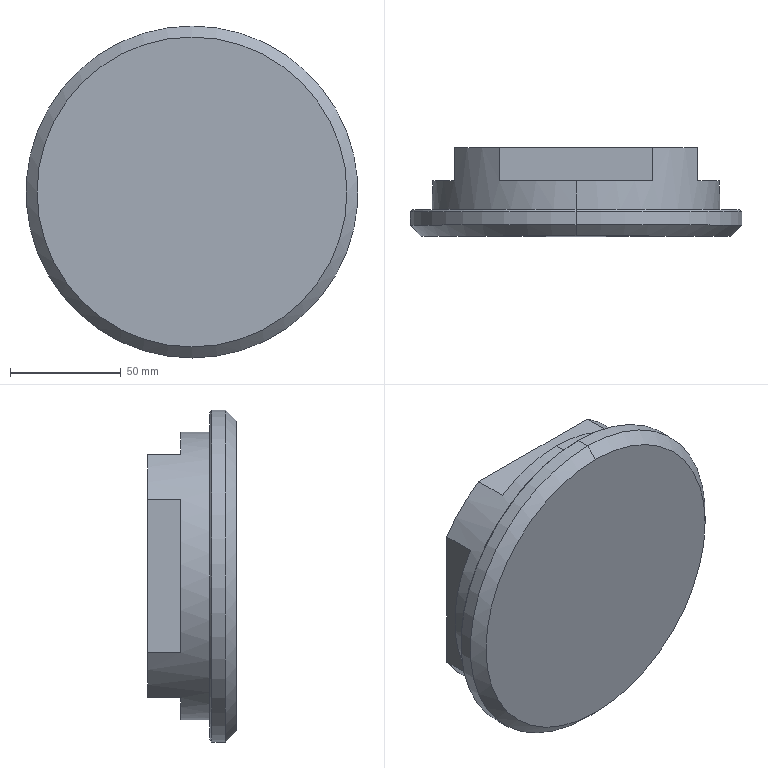Part | SolidWorks | features ICE 3, Chamfer 2, BaseBody 1 | 1 solid | 19 faces | box 150 x 40 x 150 mm | volume 549544 mm3 | plane 11 | cone 4 | cylinder 4 | commonest cylinder face diameters 130 x2 150 x2
STEP:
#1=CARTESIAN_POINT('',(0.,12.,74.));
#2=VERTEX_POINT('',#1);
#3=CARTESIAN_POINT('',(0.,12.,-74.));
#4=VERTEX_POINT('',#3);
#5=CARTESIAN_POINT('',(0.,12.,0.));
#6=DIRECTION('',(0.,1.,0.));
#7=DIRECTION('',(0.,0.,1.));
#8=AXIS2_PLACEMENT_3D('',#5,#6,#7);
#9=CIRCLE('',#8,74.);
#10=EDGE_CURVE('',#2,#4,#9,.T.);
#11=ORIENTED_EDGE('',*,*,#10,.F.);
#12=CARTESIAN_POINT('',(0.,11.,75.));
#13=VERTEX_POINT('',#12);
#14=CARTESIAN_POINT('',(0.,11.,75.));
#15=DIRECTION('',(0.,-0.7071,0.7071));
#16=VECTOR('',#15,1000.);
#17=LINE('',#14,#16);
#18=EDGE_CURVE('',#2,#13,#17,.T.);
#19=ORIENTED_EDGE('',*,*,#18,.T.);
#20=CARTESIAN_POINT('',(0.,11.,-75.));
#21=VERTEX_POINT('',#20);
#22=CARTESIAN_POINT('',(0.,11.,0.));
#23=DIRECTION('',(0.,-1.,0.));
#24=DIRECTION('',(0.,0.,1.));
#25=AXIS2_PLACEMENT_3D('',#22,#23,#24);
#26=CIRCLE('',#25,75.);
#27=EDGE_CURVE('',#21,#13,#26,.T.);
#28=ORIENTED_EDGE('',*,*,#27,.F.);
#29=CARTESIAN_POINT('',(0.,11.,-75.));
#30=DIRECTION('',(0.,-0.7071,-0.7071));
#31=VECTOR('',#30,1000.);
#32=LINE('',#29,#31);
#33=EDGE_CURVE('',#4,#21,#32,.T.);
#34=ORIENTED_EDGE('',*,*,#33,.F.);
#35=EDGE_LOOP('',(#11,#19,#28,#34));
#36=FACE_OUTER_BOUND('',#35,.T.);
#37=CARTESIAN_POINT('',(0.,11.,0.));
#38=DIRECTION('',(0.,-1.,0.));
#39=DIRECTION('',(0.,0.,-1.));
#40=AXIS2_PLACEMENT_3D('',#37,#38,#39);
#41=CONICAL_SURFACE('',#40,75.,0.7854);
#42=ADVANCED_FACE('',(#36),#41,.T.);
#43=CARTESIAN_POINT('',(0.,0.,-70.));
#44=VERTEX_POINT('',#43);
#45=CARTESIAN_POINT('',(0.,0.,70.));
#46=VERTEX_POINT('',#45);
#47=CARTESIAN_POINT('',(0.,0.,0.));
#48=DIRECTION('',(0.,-1.,0.));
#49=DIRECTION('',(0.,0.,1.));
#50=AXIS2_PLACEMENT_3D('',#47,#48,#49);
#51=CIRCLE('',#50,70.);
#52=EDGE_CURVE('',#44,#46,#51,.T.);
#53=ORIENTED_EDGE('',*,*,#52,.F.);
#54=CARTESIAN_POINT('',(0.,5.,-75.));
#55=VERTEX_POINT('',#54);
#56=CARTESIAN_POINT('',(0.,0.,-70.));
#57=DIRECTION('',(0.,0.7071,-0.7071));
#58=VECTOR('',#57,1000.);
#59=LINE('',#56,#58);
#60=EDGE_CURVE('',#44,#55,#59,.T.);
#61=ORIENTED_EDGE('',*,*,#60,.T.);
#62=CARTESIAN_POINT('',(0.,5.,75.));
#63=VERTEX_POINT('',#62);
#64=CARTESIAN_POINT('',(0.,5.,0.));
#65=DIRECTION('',(0.,1.,0.));
#66=DIRECTION('',(0.,0.,1.));
#67=AXIS2_PLACEMENT_3D('',#64,#65,#66);
#68=CIRCLE('',#67,75.);
#69=EDGE_CURVE('',#63,#55,#68,.T.);
#70=ORIENTED_EDGE('',*,*,#69,.F.);
#71=CARTESIAN_POINT('',(0.,0.,70.));
#72=DIRECTION('',(0.,0.7071,0.7071));
#73=VECTOR('',#72,1000.);
#74=LINE('',#71,#73);
#75=EDGE_CURVE('',#46,#63,#74,.T.);
#76=ORIENTED_EDGE('',*,*,#75,.F.);
#77=EDGE_LOOP('',(#53,#61,#70,#76));
#78=FACE_OUTER_BOUND('',#77,.T.);
#79=CARTESIAN_POINT('',(0.,0.,0.));
#80=DIRECTION('',(0.,1.,0.));
#81=DIRECTION('',(0.,0.,1.));
#82=AXIS2_PLACEMENT_3D('',#79,#80,#81);
#83=CONICAL_SURFACE('',#82,70.,0.7854);
#84=ADVANCED_FACE('',(#78),#83,.T.);
#85=ORIENTED_EDGE('',*,*,#27,.T.);
#86=CARTESIAN_POINT('',(0.,224.132,75.));
#87=DIRECTION('',(0.,-1.,0.));
#88=VECTOR('',#87,1000.);
#89=LINE('',#86,#88);
#90=EDGE_CURVE('',#13,#63,#89,.T.);
#91=ORIENTED_EDGE('',*,*,#90,.T.);
#92=ORIENTED_EDGE('',*,*,#69,.T.);
#93=CARTESIAN_POINT('',(0.,224.132,-75.));
#94=DIRECTION('',(0.,-1.,0.));
#95=VECTOR('',#94,1000.);
#96=LINE('',#93,#95);
#97=EDGE_CURVE('',#21,#55,#96,.T.);
#98=ORIENTED_EDGE('',*,*,#97,.F.);
#99=EDGE_LOOP('',(#85,#91,#92,#98));
#100=FACE_OUTER_BOUND('',#99,.T.);
#101=CARTESIAN_POINT('',(0.,224.132,0.));
#102=DIRECTION('',(0.,-1.,0.));
#103=DIRECTION('',(0.,0.,-1.));
#104=AXIS2_PLACEMENT_3D('',#101,#102,#103);
#105=CYLINDRICAL_SURFACE('',#104,75.);
#106=ADVANCED_FACE('',(#100),#105,.T.);
#107=CARTESIAN_POINT('',(0.,25.,65.));
#108=VERTEX_POINT('',#107);
#109=CARTESIAN_POINT('',(34.641,25.,55.));
#110=VERTEX_POINT('',#109);
#111=CARTESIAN_POINT('',(0.,25.,0.));
#112=DIRECTION('',(0.,1.,0.));
#113=DIRECTION('',(0.,0.,1.));
#114=AXIS2_PLACEMENT_3D('',#111,#112,#113);
#115=CIRCLE('',#114,65.);
#116=EDGE_CURVE('',#108,#110,#115,.T.);
#117=ORIENTED_EDGE('',*,*,#116,.F.);
#118=CARTESIAN_POINT('',(0.,12.,65.));
#119=VERTEX_POINT('',#118);
#120=CARTESIAN_POINT('',(0.,208.848,65.));
#121=DIRECTION('',(0.,-1.,0.));
#122=VECTOR('',#121,1000.);
#123=LINE('',#120,#122);
#124=EDGE_CURVE('',#108,#119,#123,.T.);
#125=ORIENTED_EDGE('',*,*,#124,.T.);
#126=CARTESIAN_POINT('',(0.,12.,-65.));
#127=VERTEX_POINT('',#126);
#128=CARTESIAN_POINT('',(0.,12.,0.));
#129=DIRECTION('',(0.,1.,0.));
#130=DIRECTION('',(0.,0.,1.));
#131=AXIS2_PLACEMENT_3D('',#128,#129,#130);
#132=CIRCLE('',#131,65.);
#133=EDGE_CURVE('',#119,#127,#132,.T.);
#134=ORIENTED_EDGE('',*,*,#133,.T.);
#135=CARTESIAN_POINT('',(0.,25.,-65.));
#136=VERTEX_POINT('',#135);
#137=CARTESIAN_POINT('',(0.,208.848,-65.));
#138=DIRECTION('',(0.,-1.,0.));
#139=VECTOR('',#138,1000.);
#140=LINE('',#137,#139);
#141=EDGE_CURVE('',#136,#127,#140,.T.);
#142=ORIENTED_EDGE('',*,*,#141,.F.);
#143=CARTESIAN_POINT('',(34.641,25.,-55.));
#144=VERTEX_POINT('',#143);
#145=CARTESIAN_POINT('',(0.,25.,0.));
#146=DIRECTION('',(0.,1.,0.));
#147=DIRECTION('',(0.,0.,1.));
#148=AXIS2_PLACEMENT_3D('',#145,#146,#147);
#149=CIRCLE('',#148,65.);
#150=EDGE_CURVE('',#144,#136,#149,.T.);
#151=ORIENTED_EDGE('',*,*,#150,.F.);
#152=CARTESIAN_POINT('',(34.641,40.,-55.));
#153=VERTEX_POINT('',#152);
#154=CARTESIAN_POINT('',(34.641,195.563,-55.));
#155=DIRECTION('',(0.,-1.,0.));
#156=VECTOR('',#155,1000.);
#157=LINE('',#154,#156);
#158=EDGE_CURVE('',#153,#144,#157,.T.);
#159=ORIENTED_EDGE('',*,*,#158,.F.);
#160=CARTESIAN_POINT('',(55.,40.,-34.641));
#161=VERTEX_POINT('',#160);
#162=CARTESIAN_POINT('',(0.,40.,0.));
#163=DIRECTION('',(0.,1.,0.));
#164=DIRECTION('',(0.,0.,1.));
#165=AXIS2_PLACEMENT_3D('',#162,#163,#164);
#166=CIRCLE('',#165,65.);
#167=EDGE_CURVE('',#161,#153,#166,.T.);
#168=ORIENTED_EDGE('',*,*,#167,.F.);
#169=CARTESIAN_POINT('',(55.,25.,-34.641));
#170=VERTEX_POINT('',#169);
#171=CARTESIAN_POINT('',(55.,195.563,-34.641));
#172=DIRECTION('',(0.,-1.,0.));
#173=VECTOR('',#172,1000.);
#174=LINE('',#171,#173);
#175=EDGE_CURVE('',#161,#170,#174,.T.);
#176=ORIENTED_EDGE('',*,*,#175,.T.);
#177=CARTESIAN_POINT('',(55.,25.,34.641));
#178=VERTEX_POINT('',#177);
#179=CARTESIAN_POINT('',(0.,25.,0.));
#180=DIRECTION('',(0.,1.,0.));
#181=DIRECTION('',(0.,0.,1.));
#182=AXIS2_PLACEMENT_3D('',#179,#180,#181);
#183=CIRCLE('',#182,65.);
#184=EDGE_CURVE('',#178,#170,#183,.T.);
#185=ORIENTED_EDGE('',*,*,#184,.F.);
#186=CARTESIAN_POINT('',(55.,40.,34.641));
#187=VERTEX_POINT('',#186);
#188=CARTESIAN_POINT('',(55.,195.563,34.641));
#189=DIRECTION('',(0.,-1.,0.));
#190=VECTOR('',#189,1000.);
#191=LINE('',#188,#190);
#192=EDGE_CURVE('',#187,#178,#191,.T.);
#193=ORIENTED_EDGE('',*,*,#192,.F.);
#194=CARTESIAN_POINT('',(34.641,40.,55.));
#195=VERTEX_POINT('',#194);
#196=CARTESIAN_POINT('',(0.,40.,0.));
#197=DIRECTION('',(0.,1.,0.));
#198=DIRECTION('',(0.,0.,1.));
#199=AXIS2_PLACEMENT_3D('',#196,#197,#198);
#200=CIRCLE('',#199,65.);
#201=EDGE_CURVE('',#195,#187,#200,.T.);
#202=ORIENTED_EDGE('',*,*,#201,.F.);
#203=CARTESIAN_POINT('',(34.641,195.563,55.));
#204=DIRECTION('',(0.,-1.,0.));
#205=VECTOR('',#204,1000.);
#206=LINE('',#203,#205);
#207=EDGE_CURVE('',#195,#110,#206,.T.);
#208=ORIENTED_EDGE('',*,*,#207,.T.);
#209=EDGE_LOOP('',(#117,#125,#134,#142,#151,#159,#168,#176,#185,#193,#202,#208));
#210=FACE_OUTER_BOUND('',#209,.T.);
#211=CARTESIAN_POINT('',(0.,208.848,0.));
#212=DIRECTION('',(0.,-1.,0.));
#213=DIRECTION('',(0.,0.,-1.));
#214=AXIS2_PLACEMENT_3D('',#211,#212,#213);
#215=CYLINDRICAL_SURFACE('',#214,65.);
#216=ADVANCED_FACE('',(#210),#215,.T.);
#217=CARTESIAN_POINT('',(-55.,25.,-34.641));
#218=VERTEX_POINT('',#217);
#219=CARTESIAN_POINT('',(-55.,25.,34.641));
#220=VERTEX_POINT('',#219);
#221=CARTESIAN_POINT('',(0.,25.,0.));
#222=DIRECTION('',(0.,1.,0.));
#223=DIRECTION('',(0.,0.,1.));
#224=AXIS2_PLACEMENT_3D('',#221,#222,#223);
#225=CIRCLE('',#224,65.);
#226=EDGE_CURVE('',#218,#220,#225,.T.);
#227=ORIENTED_EDGE('',*,*,#226,.T.);
#228=CARTESIAN_POINT('',(-55.,25.,34.641));
#229=DIRECTION('',(0.,0.,1.));
#230=VECTOR('',#229,1000.);
#231=LINE('',#228,#230);
#232=EDGE_CURVE('',#218,#220,#231,.T.);
#233=ORIENTED_EDGE('',*,*,#232,.F.);
#234=EDGE_LOOP('',(#227,#233));
#235=FACE_OUTER_BOUND('',#234,.T.);
#236=CARTESIAN_POINT('',(0.,25.,0.));
#237=DIRECTION('',(0.,1.,0.));
#238=DIRECTION('',(0.,0.,1.));
#239=AXIS2_PLACEMENT_3D('',#236,#237,#238);
#240=PLANE('',#239);
#241=ADVANCED_FACE('',(#235),#240,.T.);
#242=CARTESIAN_POINT('',(-34.641,25.,55.));
#243=VERTEX_POINT('',#242);
#244=CARTESIAN_POINT('',(0.,25.,0.));
#245=DIRECTION('',(0.,1.,0.));
#246=DIRECTION('',(0.,0.,1.));
#247=AXIS2_PLACEMENT_3D('',#244,#245,#246);
#248=CIRCLE('',#247,65.);
#249=EDGE_CURVE('',#243,#108,#248,.T.);
#250=ORIENTED_EDGE('',*,*,#249,.T.);
#251=ORIENTED_EDGE('',*,*,#116,.T.);
#252=CARTESIAN_POINT('',(-34.641,25.,55.));
#253=DIRECTION('',(1.,0.,0.));
#254=VECTOR('',#253,1000.);
#255=LINE('',#252,#254);
#256=EDGE_CURVE('',#243,#110,#255,.T.);
#257=ORIENTED_EDGE('',*,*,#256,.F.);
#258=EDGE_LOOP('',(#250,#251,#257));
#259=FACE_OUTER_BOUND('',#258,.T.);
#260=CARTESIAN_POINT('',(0.,25.,0.));
#261=DIRECTION('',(0.,1.,0.));
#262=DIRECTION('',(0.,0.,1.));
#263=AXIS2_PLACEMENT_3D('',#260,#261,#262);
#264=PLANE('',#263);
#265=ADVANCED_FACE('',(#259),#264,.T.);
#266=ORIENTED_EDGE('',*,*,#184,.T.);
#267=CARTESIAN_POINT('',(55.,25.,34.641));
#268=DIRECTION('',(0.,0.,-1.));
#269=VECTOR('',#268,1000.);
#270=LINE('',#267,#269);
#271=EDGE_CURVE('',#178,#170,#270,.T.);
#272=ORIENTED_EDGE('',*,*,#271,.F.);
#273=EDGE_LOOP('',(#266,#272));
#274=FACE_OUTER_BOUND('',#273,.T.);
#275=CARTESIAN_POINT('',(0.,25.,0.));
#276=DIRECTION('',(0.,1.,0.));
#277=DIRECTION('',(0.,0.,1.));
#278=AXIS2_PLACEMENT_3D('',#275,#276,#277);
#279=PLANE('',#278);
#280=ADVANCED_FACE('',(#274),#279,.T.);
#281=ORIENTED_EDGE('',*,*,#150,.T.);
#282=CARTESIAN_POINT('',(-34.641,25.,-55.));
#283=VERTEX_POINT('',#282);
#284=CARTESIAN_POINT('',(0.,25.,0.));
#285=DIRECTION('',(0.,1.,0.));
#286=DIRECTION('',(0.,0.,1.));
#287=AXIS2_PLACEMENT_3D('',#284,#285,#286);
#288=CIRCLE('',#287,65.);
#289=EDGE_CURVE('',#136,#283,#288,.T.);
#290=ORIENTED_EDGE('',*,*,#289,.T.);
#291=CARTESIAN_POINT('',(-34.641,25.,-55.));
#292=DIRECTION('',(-1.,0.,0.));
#293=VECTOR('',#292,1000.);
#294=LINE('',#291,#293);
#295=EDGE_CURVE('',#144,#283,#294,.T.);
#296=ORIENTED_EDGE('',*,*,#295,.F.);
#297=EDGE_LOOP('',(#281,#290,#296));
#298=FACE_OUTER_BOUND('',#297,.T.);
#299=CARTESIAN_POINT('',(0.,25.,0.));
#300=DIRECTION('',(0.,1.,0.));
#301=DIRECTION('',(0.,0.,1.));
#302=AXIS2_PLACEMENT_3D('',#299,#300,#301);
#303=PLANE('',#302);
#304=ADVANCED_FACE('',(#298),#303,.T.);
#305=ORIENTED_EDGE('',*,*,#124,.F.);
#306=ORIENTED_EDGE('',*,*,#249,.F.);
#307=CARTESIAN_POINT('',(-34.641,40.,55.));
#308=VERTEX_POINT('',#307);
#309=CARTESIAN_POINT('',(-34.641,195.563,55.));
#310=DIRECTION('',(0.,-1.,0.));
#311=VECTOR('',#310,1000.);
#312=LINE('',#309,#311);
#313=EDGE_CURVE('',#308,#243,#312,.T.);
#314=ORIENTED_EDGE('',*,*,#313,.F.);
#315=CARTESIAN_POINT('',(-55.,40.,34.641));
#316=VERTEX_POINT('',#315);
#317=CARTESIAN_POINT('',(0.,40.,0.));
#318=DIRECTION('',(0.,1.,0.));
#319=DIRECTION('',(0.,0.,1.));
#320=AXIS2_PLACEMENT_3D('',#317,#318,#319);
#321=CIRCLE('',#320,65.);
#322=EDGE_CURVE('',#316,#308,#321,.T.);
#323=ORIENTED_EDGE('',*,*,#322,.F.);
#324=CARTESIAN_POINT('',(-55.,195.563,34.641));
#325=DIRECTION('',(0.,-1.,0.));
#326=VECTOR('',#325,1000.);
#327=LINE('',#324,#326);
#328=EDGE_CURVE('',#316,#220,#327,.T.);
#329=ORIENTED_EDGE('',*,*,#328,.T.);
#330=ORIENTED_EDGE('',*,*,#226,.F.);
#331=CARTESIAN_POINT('',(-55.,40.,-34.641));
#332=VERTEX_POINT('',#331);
#333=CARTESIAN_POINT('',(-55.,195.563,-34.641));
#334=DIRECTION('',(0.,-1.,0.));
#335=VECTOR('',#334,1000.);
#336=LINE('',#333,#335);
#337=EDGE_CURVE('',#332,#218,#336,.T.);
#338=ORIENTED_EDGE('',*,*,#337,.F.);
#339=CARTESIAN_POINT('',(-34.641,40.,-55.));
#340=VERTEX_POINT('',#339);
#341=CARTESIAN_POINT('',(0.,40.,0.));
#342=DIRECTION('',(0.,1.,0.));
#343=DIRECTION('',(0.,0.,1.));
#344=AXIS2_PLACEMENT_3D('',#341,#342,#343);
#345=CIRCLE('',#344,65.);
#346=EDGE_CURVE('',#340,#332,#345,.T.);
#347=ORIENTED_EDGE('',*,*,#346,.F.);
#348=CARTESIAN_POINT('',(-34.641,195.563,-55.));
#349=DIRECTION('',(0.,-1.,0.));
#350=VECTOR('',#349,1000.);
#351=LINE('',#348,#350);
#352=EDGE_CURVE('',#340,#283,#351,.T.);
#353=ORIENTED_EDGE('',*,*,#352,.T.);
#354=ORIENTED_EDGE('',*,*,#289,.F.);
#355=ORIENTED_EDGE('',*,*,#141,.T.);
#356=CARTESIAN_POINT('',(0.,12.,0.));
#357=DIRECTION('',(0.,1.,0.));
#358=DIRECTION('',(0.,0.,1.));
#359=AXIS2_PLACEMENT_3D('',#356,#357,#358);
#360=CIRCLE('',#359,65.);
#361=EDGE_CURVE('',#127,#119,#360,.T.);
#362=ORIENTED_EDGE('',*,*,#361,.T.);
#363=EDGE_LOOP('',(#305,#306,#314,#323,#329,#330,#338,#347,#353,#354,#355,#362));
#364=FACE_OUTER_BOUND('',#363,.T.);
#365=CARTESIAN_POINT('',(0.,208.848,0.));
#366=DIRECTION('',(0.,-1.,0.));
#367=DIRECTION('',(0.,0.,-1.));
#368=AXIS2_PLACEMENT_3D('',#365,#366,#367);
#369=CYLINDRICAL_SURFACE('',#368,65.);
#370=ADVANCED_FACE('',(#364),#369,.T.);
#371=CARTESIAN_POINT('',(0.,12.,0.));
#372=DIRECTION('',(0.,1.,0.));
#373=DIRECTION('',(0.,0.,1.));
#374=AXIS2_PLACEMENT_3D('',#371,#372,#373);
#375=CIRCLE('',#374,74.);
#376=EDGE_CURVE('',#4,#2,#375,.T.);
#377=ORIENTED_EDGE('',*,*,#376,.T.);
#378=ORIENTED_EDGE('',*,*,#10,.T.);
#379=EDGE_LOOP('',(#377,#378));
#380=FACE_OUTER_BOUND('',#379,.T.);
#381=ORIENTED_EDGE('',*,*,#361,.F.);
#382=ORIENTED_EDGE('',*,*,#133,.F.);
#383=EDGE_LOOP('',(#381,#382));
#384=FACE_BOUND('',#383,.T.);
#385=CARTESIAN_POINT('',(0.,12.,0.));
#386=DIRECTION('',(0.,1.,0.));
#387=DIRECTION('',(0.,0.,1.));
#388=AXIS2_PLACEMENT_3D('',#385,#386,#387);
#389=PLANE('',#388);
#390=ADVANCED_FACE('',(#380,#384),#389,.T.);
#391=ORIENTED_EDGE('',*,*,#90,.F.);
#392=CARTESIAN_POINT('',(0.,11.,0.));
#393=DIRECTION('',(0.,-1.,0.));
#394=DIRECTION('',(0.,0.,1.));
#395=AXIS2_PLACEMENT_3D('',#392,#393,#394);
#396=CIRCLE('',#395,75.);
#397=EDGE_CURVE('',#13,#21,#396,.T.);
#398=ORIENTED_EDGE('',*,*,#397,.T.);
#399=ORIENTED_EDGE('',*,*,#97,.T.);
#400=CARTESIAN_POINT('',(0.,5.,0.));
#401=DIRECTION('',(0.,1.,0.));
#402=DIRECTION('',(0.,0.,1.));
#403=AXIS2_PLACEMENT_3D('',#400,#401,#402);
#404=CIRCLE('',#403,75.);
#405=EDGE_CURVE('',#55,#63,#404,.T.);
#406=ORIENTED_EDGE('',*,*,#405,.T.);
#407=EDGE_LOOP('',(#391,#398,#399,#406));
#408=FACE_OUTER_BOUND('',#407,.T.);
#409=CARTESIAN_POINT('',(0.,224.132,0.));
#410=DIRECTION('',(0.,-1.,0.));
#411=DIRECTION('',(0.,0.,-1.));
#412=AXIS2_PLACEMENT_3D('',#409,#410,#411);
#413=CYLINDRICAL_SURFACE('',#412,75.);
#414=ADVANCED_FACE('',(#408),#413,.T.);
#415=CARTESIAN_POINT('',(0.,0.,0.));
#416=DIRECTION('',(0.,-1.,0.));
#417=DIRECTION('',(0.,0.,1.));
#418=AXIS2_PLACEMENT_3D('',#415,#416,#417);
#419=CIRCLE('',#418,70.);
#420=EDGE_CURVE('',#46,#44,#419,.T.);
#421=ORIENTED_EDGE('',*,*,#420,.T.);
#422=ORIENTED_EDGE('',*,*,#52,.T.);
#423=EDGE_LOOP('',(#421,#422));
#424=FACE_OUTER_BOUND('',#423,.T.);
#425=CARTESIAN_POINT('',(0.,0.,0.));
#426=DIRECTION('',(0.,1.,0.));
#427=DIRECTION('',(0.,0.,1.));
#428=AXIS2_PLACEMENT_3D('',#425,#426,#427);
#429=PLANE('',#428);
#430=ADVANCED_FACE('',(#424),#429,.F.);
#431=CARTESIAN_POINT('',(-34.641,40.,-55.));
#432=DIRECTION('',(-1.,0.,0.));
#433=VECTOR('',#432,1000.);
#434=LINE('',#431,#433);
#435=EDGE_CURVE('',#153,#340,#434,.T.);
#436=ORIENTED_EDGE('',*,*,#435,.F.);
#437=ORIENTED_EDGE('',*,*,#158,.T.);
#438=ORIENTED_EDGE('',*,*,#295,.T.);
#439=ORIENTED_EDGE('',*,*,#352,.F.);
#440=EDGE_LOOP('',(#436,#437,#438,#439));
#441=FACE_OUTER_BOUND('',#440,.T.);
#442=CARTESIAN_POINT('',(-34.641,195.563,-55.));
#443=DIRECTION('',(0.,0.,1.));
#444=DIRECTION('',(1.,0.,0.));
#445=AXIS2_PLACEMENT_3D('',#442,#443,#444);
#446=PLANE('',#445);
#447=ADVANCED_FACE('',(#441),#446,.F.);
#448=CARTESIAN_POINT('',(55.,40.,34.641));
#449=DIRECTION('',(0.,0.,-1.));
#450=VECTOR('',#449,1000.);
#451=LINE('',#448,#450);
#452=EDGE_CURVE('',#187,#161,#451,.T.);
#453=ORIENTED_EDGE('',*,*,#452,.F.);
#454=ORIENTED_EDGE('',*,*,#192,.T.);
#455=ORIENTED_EDGE('',*,*,#271,.T.);
#456=ORIENTED_EDGE('',*,*,#175,.F.);
#457=EDGE_LOOP('',(#453,#454,#455,#456));
#458=FACE_OUTER_BOUND('',#457,.T.);
#459=CARTESIAN_POINT('',(55.,195.563,34.641));
#460=DIRECTION('',(-1.,0.,0.));
#461=DIRECTION('',(0.,0.,1.));
#462=AXIS2_PLACEMENT_3D('',#459,#460,#461);
#463=PLANE('',#462);
#464=ADVANCED_FACE('',(#458),#463,.F.);
#465=CARTESIAN_POINT('',(-34.641,40.,55.));
#466=DIRECTION('',(1.,0.,0.));
#467=VECTOR('',#466,1000.);
#468=LINE('',#465,#467);
#469=EDGE_CURVE('',#308,#195,#468,.T.);
#470=ORIENTED_EDGE('',*,*,#469,.F.);
#471=ORIENTED_EDGE('',*,*,#313,.T.);
#472=ORIENTED_EDGE('',*,*,#256,.T.);
#473=ORIENTED_EDGE('',*,*,#207,.F.);
#474=EDGE_LOOP('',(#470,#471,#472,#473));
#475=FACE_OUTER_BOUND('',#474,.T.);
#476=CARTESIAN_POINT('',(-34.641,195.563,55.));
#477=DIRECTION('',(0.,0.,-1.));
#478=DIRECTION('',(-1.,0.,0.));
#479=AXIS2_PLACEMENT_3D('',#476,#477,#478);
#480=PLANE('',#479);
#481=ADVANCED_FACE('',(#475),#480,.F.);
#482=CARTESIAN_POINT('',(-55.,40.,34.641));
#483=DIRECTION('',(0.,0.,1.));
#484=VECTOR('',#483,1000.);
#485=LINE('',#482,#484);
#486=EDGE_CURVE('',#332,#316,#485,.T.);
#487=ORIENTED_EDGE('',*,*,#486,.F.);
#488=ORIENTED_EDGE('',*,*,#337,.T.);
#489=ORIENTED_EDGE('',*,*,#232,.T.);
#490=ORIENTED_EDGE('',*,*,#328,.F.);
#491=EDGE_LOOP('',(#487,#488,#489,#490));
#492=FACE_OUTER_BOUND('',#491,.T.);
#493=CARTESIAN_POINT('',(-55.,195.563,34.641));
#494=DIRECTION('',(1.,0.,0.));
#495=DIRECTION('',(0.,0.,-1.));
#496=AXIS2_PLACEMENT_3D('',#493,#494,#495);
#497=PLANE('',#496);
#498=ADVANCED_FACE('',(#492),#497,.F.);
#499=ORIENTED_EDGE('',*,*,#435,.T.);
#500=ORIENTED_EDGE('',*,*,#346,.T.);
#501=ORIENTED_EDGE('',*,*,#486,.T.);
#502=ORIENTED_EDGE('',*,*,#322,.T.);
#503=ORIENTED_EDGE('',*,*,#469,.T.);
#504=ORIENTED_EDGE('',*,*,#201,.T.);
#505=ORIENTED_EDGE('',*,*,#452,.T.);
#506=ORIENTED_EDGE('',*,*,#167,.T.);
#507=EDGE_LOOP('',(#499,#500,#501,#502,#503,#504,#505,#506));
#508=FACE_OUTER_BOUND('',#507,.T.);
#509=CARTESIAN_POINT('',(0.,40.,0.));
#510=DIRECTION('',(0.,1.,0.));
#511=DIRECTION('',(0.,0.,1.));
#512=AXIS2_PLACEMENT_3D('',#509,#510,#511);
#513=PLANE('',#512);
#514=ADVANCED_FACE('',(#508),#513,.T.);
#515=ORIENTED_EDGE('',*,*,#60,.F.);
#516=ORIENTED_EDGE('',*,*,#420,.F.);
#517=ORIENTED_EDGE('',*,*,#75,.T.);
#518=ORIENTED_EDGE('',*,*,#405,.F.);
#519=EDGE_LOOP('',(#515,#516,#517,#518));
#520=FACE_OUTER_BOUND('',#519,.T.);
#521=CARTESIAN_POINT('',(0.,0.,0.));
#522=DIRECTION('',(0.,1.,0.));
#523=DIRECTION('',(0.,0.,1.));
#524=AXIS2_PLACEMENT_3D('',#521,#522,#523);
#525=CONICAL_SURFACE('',#524,70.,0.7854);
#526=ADVANCED_FACE('',(#520),#525,.T.);
#527=ORIENTED_EDGE('',*,*,#18,.F.);
#528=ORIENTED_EDGE('',*,*,#376,.F.);
#529=ORIENTED_EDGE('',*,*,#33,.T.);
#530=ORIENTED_EDGE('',*,*,#397,.F.);
#531=EDGE_LOOP('',(#527,#528,#529,#530));
#532=FACE_OUTER_BOUND('',#531,.T.);
#533=CARTESIAN_POINT('',(0.,11.,0.));
#534=DIRECTION('',(0.,-1.,0.));
#535=DIRECTION('',(0.,0.,-1.));
#536=AXIS2_PLACEMENT_3D('',#533,#534,#535);
#537=CONICAL_SURFACE('',#536,75.,0.7854);
#538=ADVANCED_FACE('',(#532),#537,.T.);
#539=CLOSED_SHELL('',(#42,#84,#106,#216,#241,#265,#280,#304,#370,#390,#414,#430,#447,#464,#481,#498,#514,#526,#538));
#540=MANIFOLD_SOLID_BREP('',#539);
#541=CARTESIAN_POINT('',(0.,0.,0.));
#542=DIRECTION('',(0.,0.,1.));
#543=DIRECTION('',(1.,0.,0.));
#544=AXIS2_PLACEMENT_3D('',#541,#542,#543);
#545=(LENGTH_UNIT()NAMED_UNIT(*)SI_UNIT(.MILLI.,.METRE.));
#546=UNCERTAINTY_MEASURE_WITH_UNIT(LENGTH_MEASURE(0.00001),#545,'','');
#547=(NAMED_UNIT(*)PLANE_ANGLE_UNIT()SI_UNIT($,.RADIAN.));
#548=(NAMED_UNIT(*)SI_UNIT($,.STERADIAN.)SOLID_ANGLE_UNIT());
#549=(GEOMETRIC_REPRESENTATION_CONTEXT(3)GLOBAL_UNCERTAINTY_ASSIGNED_CONTEXT((#546))GLOBAL_UNIT_ASSIGNED_CONTEXT((#545,#547,#548))REPRESENTATION_CONTEXT('',''));
#550=ADVANCED_BREP_SHAPE_REPRESENTATION('',(#540,#544),#549);